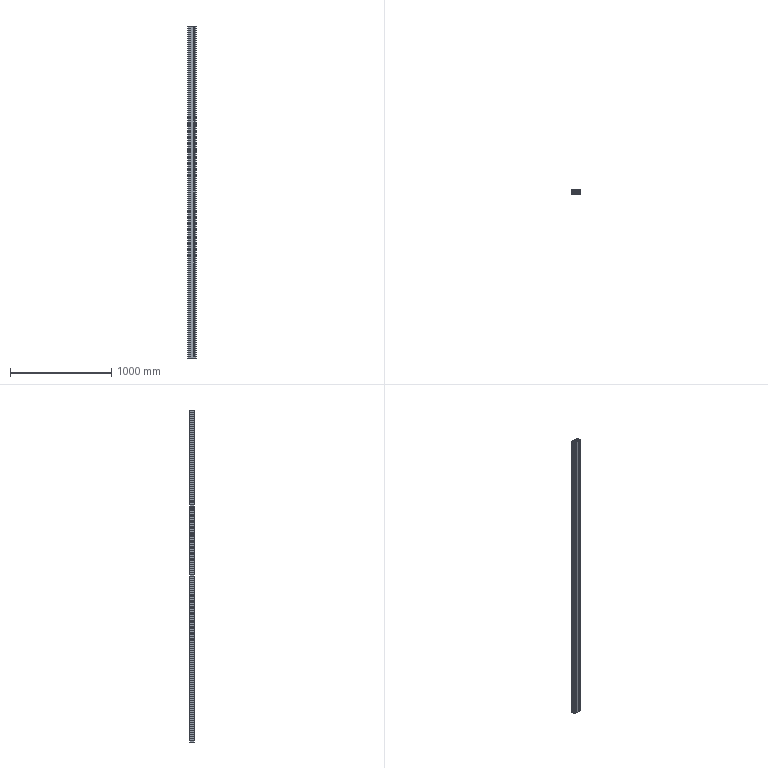Part | 1 solid | 384 faces | box 80 x 40 x 3280 mm | volume 3587950 mm3 | plane 262 | cylinder 122 | commonest cylinder face diameters 6.6 x32 6.8 x18 0.6 x16 11 x16 1 x12 1.5 x12